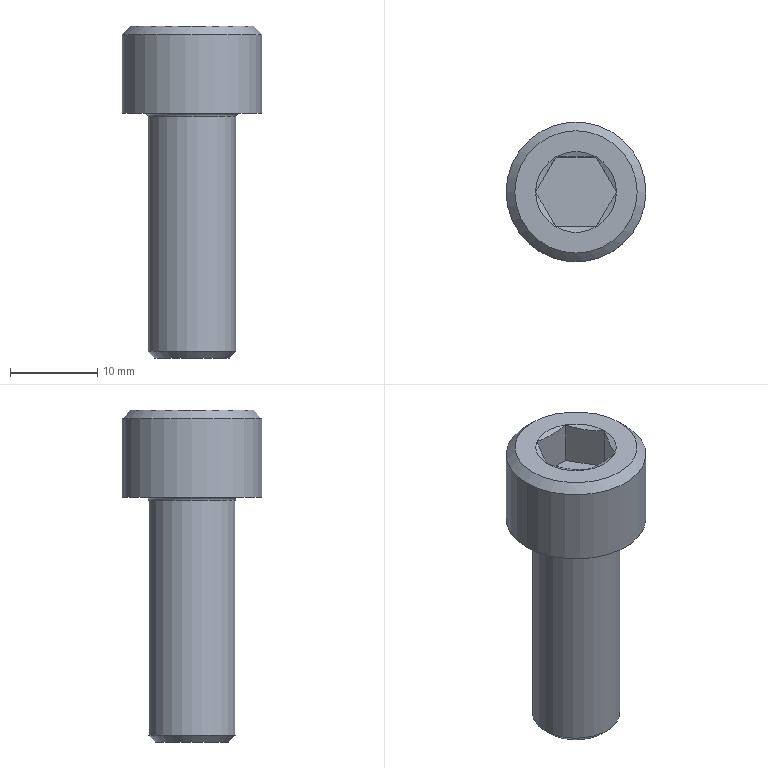Part | STEP file | solid 115 | 1 solid | 21 faces | box 16 x 16 x 38 mm | volume 3900 mm3 | plane 10 | sphere 6 | cylinder 2 | cone 2 | torus 1 | commonest cylinder face diameters 10 x1 16 x1